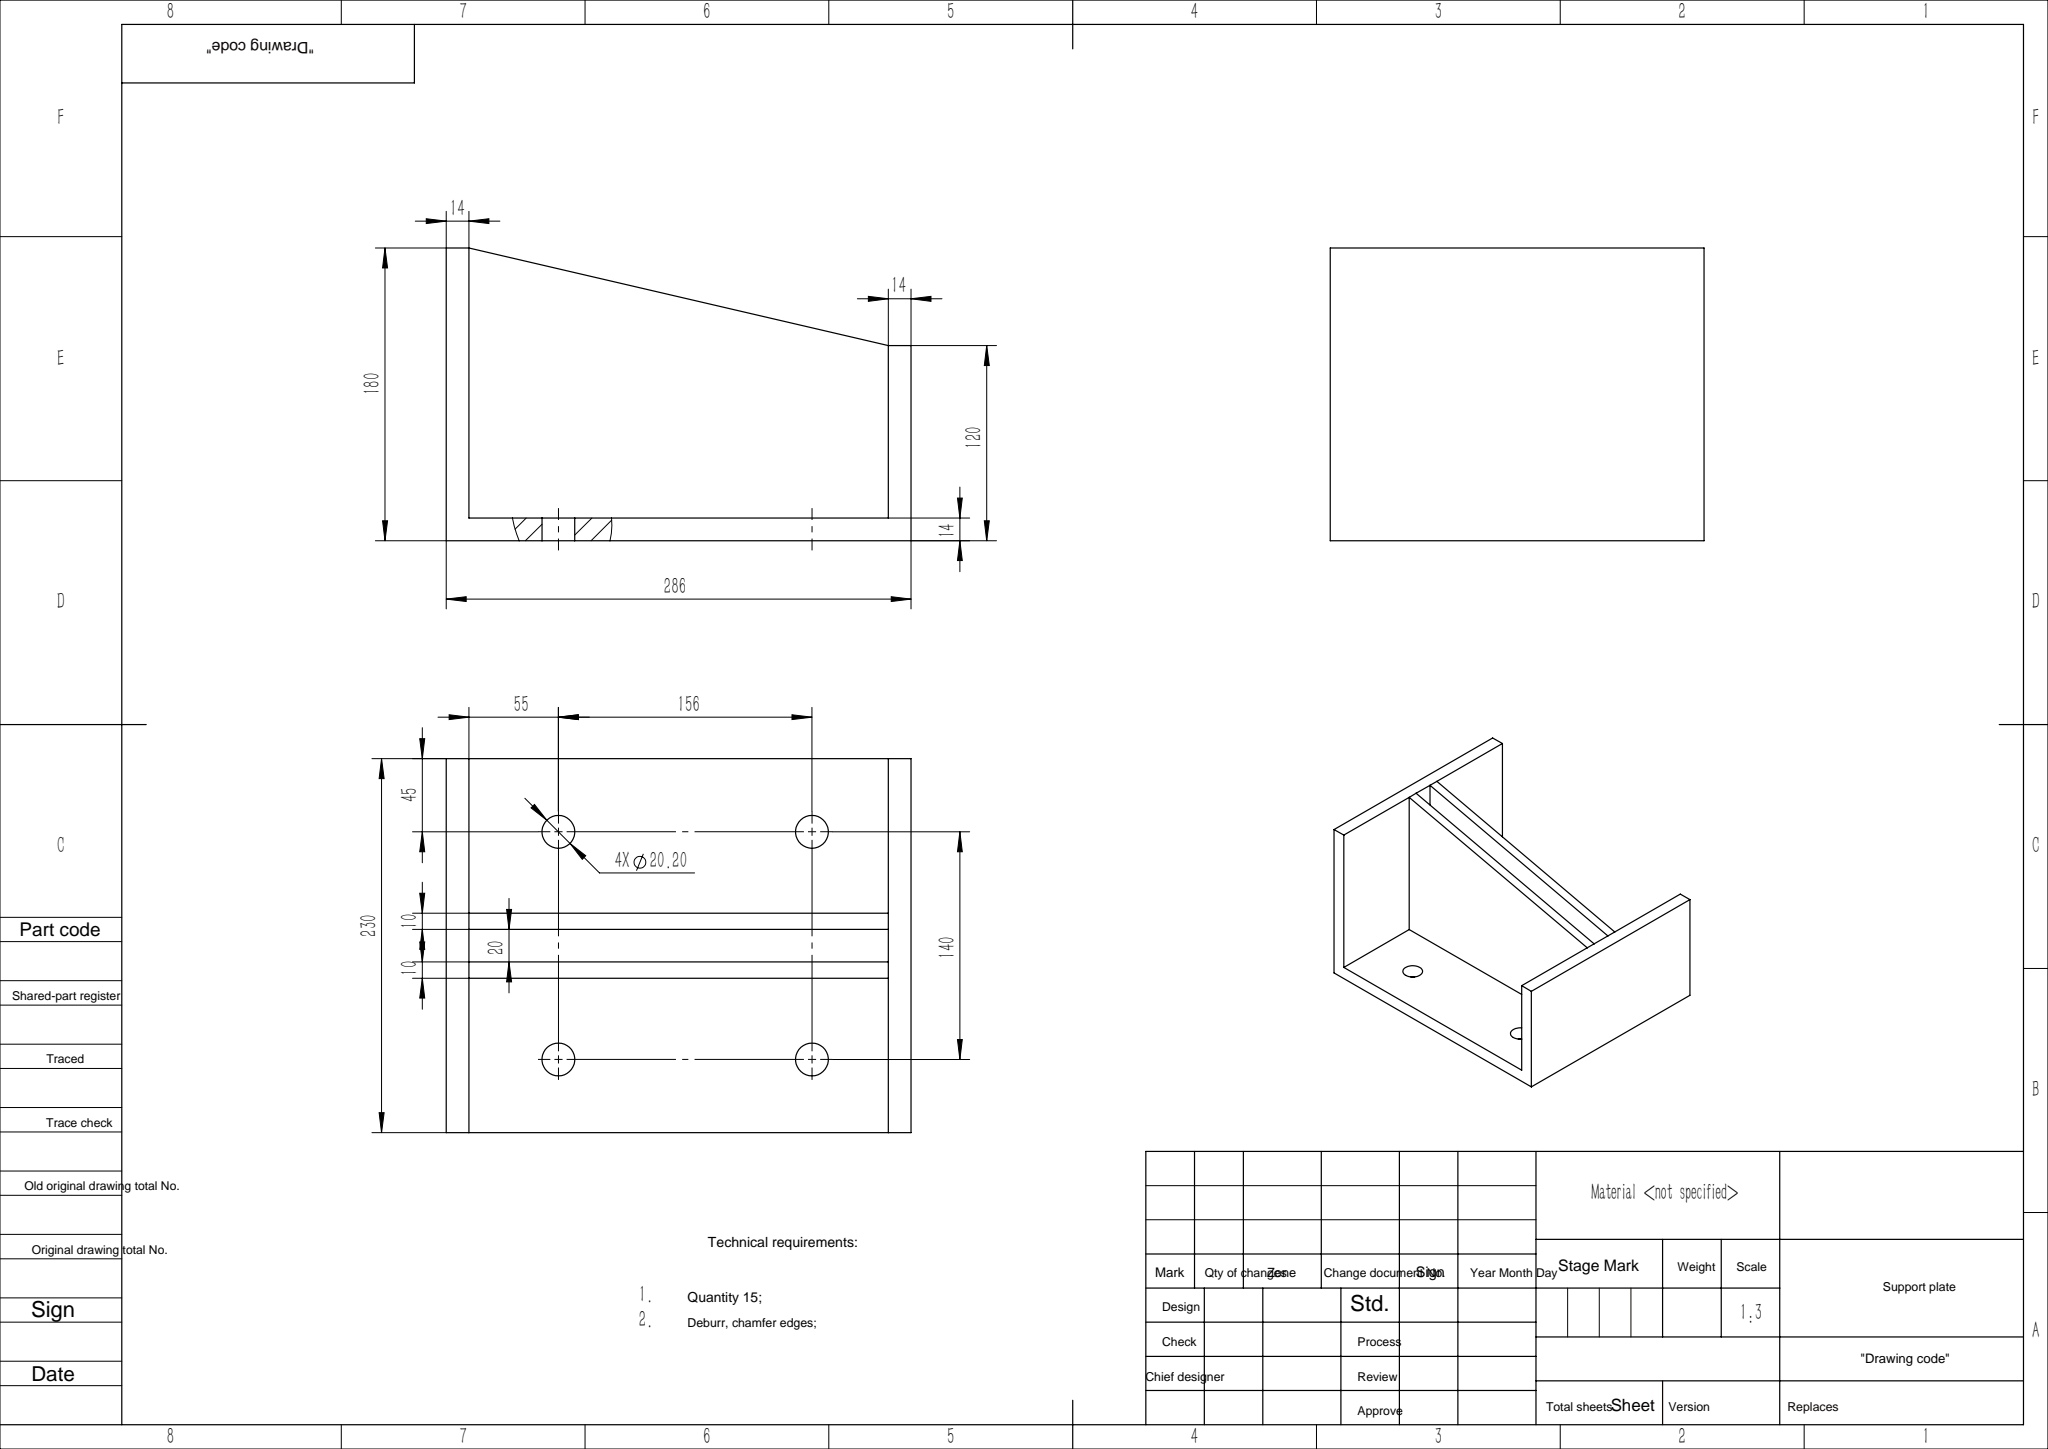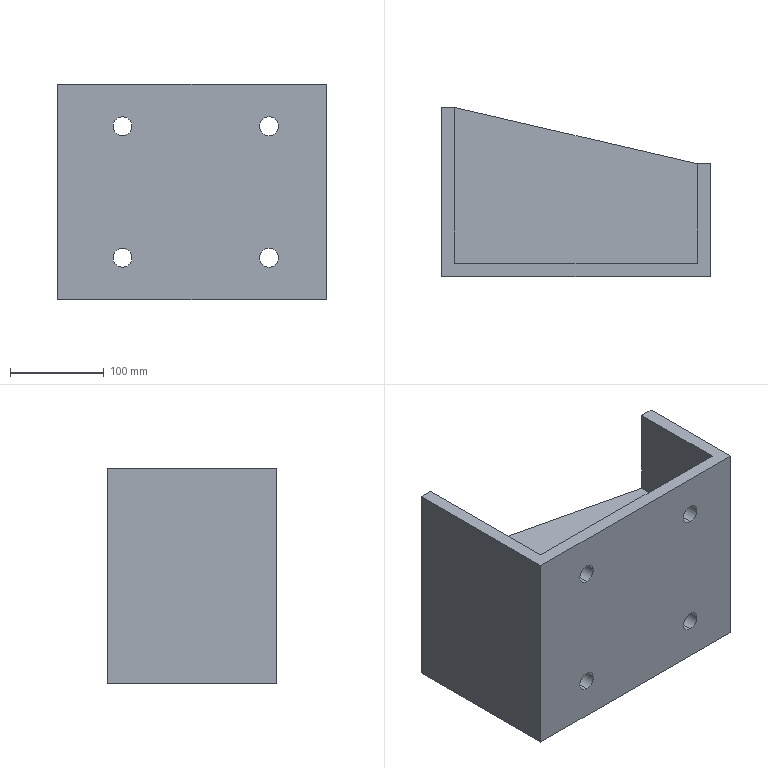Part | SolidWorks | features ICE 3, Extrusion 1, LPattern 1 | 1 solid | 30 faces | box 286 x 180 x 230 mm | volume 2480573 mm3 | plane 22 | cylinder 8 | commonest cylinder face diameters 20.2 x8
STEP:
#1=CARTESIAN_POINT('',(82.,0.,59.9));
#2=VERTEX_POINT('',#1);
#3=CARTESIAN_POINT('',(82.,0.,80.1));
#4=VERTEX_POINT('',#3);
#5=CARTESIAN_POINT('',(82.,0.,70.));
#6=DIRECTION('',(0.,1.,0.));
#7=DIRECTION('',(0.,0.,1.));
#8=AXIS2_PLACEMENT_3D('',#5,#6,#7);
#9=CIRCLE('',#8,10.1);
#10=EDGE_CURVE('',#2,#4,#9,.T.);
#11=ORIENTED_EDGE('',*,*,#10,.F.);
#12=CARTESIAN_POINT('',(82.,14.,59.9));
#13=VERTEX_POINT('',#12);
#14=CARTESIAN_POINT('',(82.,0.,59.9));
#15=DIRECTION('',(0.,1.,0.));
#16=VECTOR('',#15,1000.);
#17=LINE('',#14,#16);
#18=EDGE_CURVE('',#2,#13,#17,.T.);
#19=ORIENTED_EDGE('',*,*,#18,.T.);
#20=CARTESIAN_POINT('',(82.,14.,80.1));
#21=VERTEX_POINT('',#20);
#22=CARTESIAN_POINT('',(82.,14.,70.));
#23=DIRECTION('',(0.,1.,0.));
#24=DIRECTION('',(0.,0.,1.));
#25=AXIS2_PLACEMENT_3D('',#22,#23,#24);
#26=CIRCLE('',#25,10.1);
#27=EDGE_CURVE('',#13,#21,#26,.T.);
#28=ORIENTED_EDGE('',*,*,#27,.T.);
#29=CARTESIAN_POINT('',(82.,0.,80.1));
#30=DIRECTION('',(0.,1.,0.));
#31=VECTOR('',#30,1000.);
#32=LINE('',#29,#31);
#33=EDGE_CURVE('',#4,#21,#32,.T.);
#34=ORIENTED_EDGE('',*,*,#33,.F.);
#35=EDGE_LOOP('',(#11,#19,#28,#34));
#36=FACE_OUTER_BOUND('',#35,.T.);
#37=CARTESIAN_POINT('',(82.,0.,70.));
#38=DIRECTION('',(0.,1.,0.));
#39=DIRECTION('',(0.,0.,1.));
#40=AXIS2_PLACEMENT_3D('',#37,#38,#39);
#41=CYLINDRICAL_SURFACE('',#40,10.1);
#42=ADVANCED_FACE('',(#36),#41,.F.);
#43=CARTESIAN_POINT('',(82.,0.,-80.1));
#44=VERTEX_POINT('',#43);
#45=CARTESIAN_POINT('',(82.,0.,-59.9));
#46=VERTEX_POINT('',#45);
#47=CARTESIAN_POINT('',(82.,0.,-70.));
#48=DIRECTION('',(0.,1.,0.));
#49=DIRECTION('',(0.,0.,1.));
#50=AXIS2_PLACEMENT_3D('',#47,#48,#49);
#51=CIRCLE('',#50,10.1);
#52=EDGE_CURVE('',#44,#46,#51,.T.);
#53=ORIENTED_EDGE('',*,*,#52,.F.);
#54=CARTESIAN_POINT('',(82.,14.,-80.1));
#55=VERTEX_POINT('',#54);
#56=CARTESIAN_POINT('',(82.,0.,-80.1));
#57=DIRECTION('',(0.,1.,0.));
#58=VECTOR('',#57,1000.);
#59=LINE('',#56,#58);
#60=EDGE_CURVE('',#44,#55,#59,.T.);
#61=ORIENTED_EDGE('',*,*,#60,.T.);
#62=CARTESIAN_POINT('',(82.,14.,-59.9));
#63=VERTEX_POINT('',#62);
#64=CARTESIAN_POINT('',(82.,14.,-70.));
#65=DIRECTION('',(0.,1.,0.));
#66=DIRECTION('',(0.,0.,1.));
#67=AXIS2_PLACEMENT_3D('',#64,#65,#66);
#68=CIRCLE('',#67,10.1);
#69=EDGE_CURVE('',#55,#63,#68,.T.);
#70=ORIENTED_EDGE('',*,*,#69,.T.);
#71=CARTESIAN_POINT('',(82.,0.,-59.9));
#72=DIRECTION('',(0.,1.,0.));
#73=VECTOR('',#72,1000.);
#74=LINE('',#71,#73);
#75=EDGE_CURVE('',#46,#63,#74,.T.);
#76=ORIENTED_EDGE('',*,*,#75,.F.);
#77=EDGE_LOOP('',(#53,#61,#70,#76));
#78=FACE_OUTER_BOUND('',#77,.T.);
#79=CARTESIAN_POINT('',(82.,0.,-70.));
#80=DIRECTION('',(0.,1.,0.));
#81=DIRECTION('',(0.,0.,1.));
#82=AXIS2_PLACEMENT_3D('',#79,#80,#81);
#83=CYLINDRICAL_SURFACE('',#82,10.1);
#84=ADVANCED_FACE('',(#78),#83,.F.);
#85=CARTESIAN_POINT('',(-74.,0.,-80.1));
#86=VERTEX_POINT('',#85);
#87=CARTESIAN_POINT('',(-74.,0.,-59.9));
#88=VERTEX_POINT('',#87);
#89=CARTESIAN_POINT('',(-74.,0.,-70.));
#90=DIRECTION('',(0.,1.,0.));
#91=DIRECTION('',(0.,0.,1.));
#92=AXIS2_PLACEMENT_3D('',#89,#90,#91);
#93=CIRCLE('',#92,10.1);
#94=EDGE_CURVE('',#86,#88,#93,.T.);
#95=ORIENTED_EDGE('',*,*,#94,.F.);
#96=CARTESIAN_POINT('',(-74.,14.,-80.1));
#97=VERTEX_POINT('',#96);
#98=CARTESIAN_POINT('',(-74.,0.,-80.1));
#99=DIRECTION('',(0.,1.,0.));
#100=VECTOR('',#99,1000.);
#101=LINE('',#98,#100);
#102=EDGE_CURVE('',#86,#97,#101,.T.);
#103=ORIENTED_EDGE('',*,*,#102,.T.);
#104=CARTESIAN_POINT('',(-74.,14.,-59.9));
#105=VERTEX_POINT('',#104);
#106=CARTESIAN_POINT('',(-74.,14.,-70.));
#107=DIRECTION('',(0.,1.,0.));
#108=DIRECTION('',(0.,0.,1.));
#109=AXIS2_PLACEMENT_3D('',#106,#107,#108);
#110=CIRCLE('',#109,10.1);
#111=EDGE_CURVE('',#97,#105,#110,.T.);
#112=ORIENTED_EDGE('',*,*,#111,.T.);
#113=CARTESIAN_POINT('',(-74.,0.,-59.9));
#114=DIRECTION('',(0.,1.,0.));
#115=VECTOR('',#114,1000.);
#116=LINE('',#113,#115);
#117=EDGE_CURVE('',#88,#105,#116,.T.);
#118=ORIENTED_EDGE('',*,*,#117,.F.);
#119=EDGE_LOOP('',(#95,#103,#112,#118));
#120=FACE_OUTER_BOUND('',#119,.T.);
#121=CARTESIAN_POINT('',(-74.,0.,-70.));
#122=DIRECTION('',(0.,1.,0.));
#123=DIRECTION('',(0.,0.,1.));
#124=AXIS2_PLACEMENT_3D('',#121,#122,#123);
#125=CYLINDRICAL_SURFACE('',#124,10.1);
#126=ADVANCED_FACE('',(#120),#125,.F.);
#127=CARTESIAN_POINT('',(-74.,0.,59.9));
#128=VERTEX_POINT('',#127);
#129=CARTESIAN_POINT('',(-74.,0.,80.1));
#130=VERTEX_POINT('',#129);
#131=CARTESIAN_POINT('',(-74.,0.,70.));
#132=DIRECTION('',(0.,1.,0.));
#133=DIRECTION('',(0.,0.,1.));
#134=AXIS2_PLACEMENT_3D('',#131,#132,#133);
#135=CIRCLE('',#134,10.1);
#136=EDGE_CURVE('',#128,#130,#135,.T.);
#137=ORIENTED_EDGE('',*,*,#136,.F.);
#138=CARTESIAN_POINT('',(-74.,14.,59.9));
#139=VERTEX_POINT('',#138);
#140=CARTESIAN_POINT('',(-74.,0.,59.9));
#141=DIRECTION('',(0.,1.,0.));
#142=VECTOR('',#141,1000.);
#143=LINE('',#140,#142);
#144=EDGE_CURVE('',#128,#139,#143,.T.);
#145=ORIENTED_EDGE('',*,*,#144,.T.);
#146=CARTESIAN_POINT('',(-74.,14.,80.1));
#147=VERTEX_POINT('',#146);
#148=CARTESIAN_POINT('',(-74.,14.,70.));
#149=DIRECTION('',(0.,1.,0.));
#150=DIRECTION('',(0.,0.,1.));
#151=AXIS2_PLACEMENT_3D('',#148,#149,#150);
#152=CIRCLE('',#151,10.1);
#153=EDGE_CURVE('',#139,#147,#152,.T.);
#154=ORIENTED_EDGE('',*,*,#153,.T.);
#155=CARTESIAN_POINT('',(-74.,0.,80.1));
#156=DIRECTION('',(0.,1.,0.));
#157=VECTOR('',#156,1000.);
#158=LINE('',#155,#157);
#159=EDGE_CURVE('',#130,#147,#158,.T.);
#160=ORIENTED_EDGE('',*,*,#159,.F.);
#161=EDGE_LOOP('',(#137,#145,#154,#160));
#162=FACE_OUTER_BOUND('',#161,.T.);
#163=CARTESIAN_POINT('',(-74.,0.,70.));
#164=DIRECTION('',(0.,1.,0.));
#165=DIRECTION('',(0.,0.,1.));
#166=AXIS2_PLACEMENT_3D('',#163,#164,#165);
#167=CYLINDRICAL_SURFACE('',#166,10.1);
#168=ADVANCED_FACE('',(#162),#167,.F.);
#169=CARTESIAN_POINT('',(129.,14.,10.));
#170=VERTEX_POINT('',#169);
#171=CARTESIAN_POINT('',(129.,120.,10.));
#172=VERTEX_POINT('',#171);
#173=CARTESIAN_POINT('',(129.,14.,10.));
#174=DIRECTION('',(0.,1.,0.));
#175=VECTOR('',#174,1000.);
#176=LINE('',#173,#175);
#177=EDGE_CURVE('',#170,#172,#176,.T.);
#178=ORIENTED_EDGE('',*,*,#177,.T.);
#179=CARTESIAN_POINT('',(129.,120.,-10.));
#180=VERTEX_POINT('',#179);
#181=CARTESIAN_POINT('',(129.,120.,115.));
#182=DIRECTION('',(0.,0.,-1.));
#183=VECTOR('',#182,1000.);
#184=LINE('',#181,#183);
#185=EDGE_CURVE('',#172,#180,#184,.T.);
#186=ORIENTED_EDGE('',*,*,#185,.T.);
#187=CARTESIAN_POINT('',(129.,14.,-10.));
#188=VERTEX_POINT('',#187);
#189=CARTESIAN_POINT('',(129.,120.,-10.));
#190=DIRECTION('',(0.,1.,0.));
#191=VECTOR('',#190,1000.);
#192=LINE('',#189,#191);
#193=EDGE_CURVE('',#188,#180,#192,.T.);
#194=ORIENTED_EDGE('',*,*,#193,.F.);
#195=CARTESIAN_POINT('',(129.,14.,115.));
#196=DIRECTION('',(0.,0.,-1.));
#197=VECTOR('',#196,1000.);
#198=LINE('',#195,#197);
#199=EDGE_CURVE('',#170,#188,#198,.T.);
#200=ORIENTED_EDGE('',*,*,#199,.F.);
#201=EDGE_LOOP('',(#178,#186,#194,#200));
#202=FACE_OUTER_BOUND('',#201,.T.);
#203=CARTESIAN_POINT('',(129.,14.,115.));
#204=DIRECTION('',(1.,0.,0.));
#205=DIRECTION('',(0.,1.,0.));
#206=AXIS2_PLACEMENT_3D('',#203,#204,#205);
#207=PLANE('',#206);
#208=ADVANCED_FACE('',(#202),#207,.F.);
#209=CARTESIAN_POINT('',(-129.,14.,10.));
#210=VERTEX_POINT('',#209);
#211=CARTESIAN_POINT('',(-129.,14.,10.));
#212=DIRECTION('',(1.,0.,0.));
#213=VECTOR('',#212,1000.);
#214=LINE('',#211,#213);
#215=EDGE_CURVE('',#210,#170,#214,.T.);
#216=ORIENTED_EDGE('',*,*,#215,.T.);
#217=ORIENTED_EDGE('',*,*,#199,.T.);
#218=CARTESIAN_POINT('',(-129.,14.,-10.));
#219=VERTEX_POINT('',#218);
#220=CARTESIAN_POINT('',(129.,14.,-10.));
#221=DIRECTION('',(1.,0.,0.));
#222=VECTOR('',#221,1000.);
#223=LINE('',#220,#222);
#224=EDGE_CURVE('',#219,#188,#223,.T.);
#225=ORIENTED_EDGE('',*,*,#224,.F.);
#226=CARTESIAN_POINT('',(-129.,14.,115.));
#227=DIRECTION('',(0.,0.,-1.));
#228=VECTOR('',#227,1000.);
#229=LINE('',#226,#228);
#230=EDGE_CURVE('',#210,#219,#229,.T.);
#231=ORIENTED_EDGE('',*,*,#230,.F.);
#232=EDGE_LOOP('',(#216,#217,#225,#231));
#233=FACE_OUTER_BOUND('',#232,.T.);
#234=CARTESIAN_POINT('',(-129.,14.,115.));
#235=DIRECTION('',(0.,-1.,0.));
#236=DIRECTION('',(0.,0.,-1.));
#237=AXIS2_PLACEMENT_3D('',#234,#235,#236);
#238=PLANE('',#237);
#239=ADVANCED_FACE('',(#233),#238,.F.);
#240=CARTESIAN_POINT('',(-129.,180.,10.));
#241=VERTEX_POINT('',#240);
#242=CARTESIAN_POINT('',(-129.,180.,10.));
#243=DIRECTION('',(0.,-1.,0.));
#244=VECTOR('',#243,1000.);
#245=LINE('',#242,#244);
#246=EDGE_CURVE('',#241,#210,#245,.T.);
#247=ORIENTED_EDGE('',*,*,#246,.T.);
#248=ORIENTED_EDGE('',*,*,#230,.T.);
#249=CARTESIAN_POINT('',(-129.,180.,-10.));
#250=VERTEX_POINT('',#249);
#251=CARTESIAN_POINT('',(-129.,14.,-10.));
#252=DIRECTION('',(0.,-1.,0.));
#253=VECTOR('',#252,1000.);
#254=LINE('',#251,#253);
#255=EDGE_CURVE('',#250,#219,#254,.T.);
#256=ORIENTED_EDGE('',*,*,#255,.F.);
#257=CARTESIAN_POINT('',(-129.,180.,115.));
#258=DIRECTION('',(0.,0.,-1.));
#259=VECTOR('',#258,1000.);
#260=LINE('',#257,#259);
#261=EDGE_CURVE('',#241,#250,#260,.T.);
#262=ORIENTED_EDGE('',*,*,#261,.F.);
#263=EDGE_LOOP('',(#247,#248,#256,#262));
#264=FACE_OUTER_BOUND('',#263,.T.);
#265=CARTESIAN_POINT('',(-129.,180.,115.));
#266=DIRECTION('',(-1.,0.,0.));
#267=DIRECTION('',(0.,-1.,0.));
#268=AXIS2_PLACEMENT_3D('',#265,#266,#267);
#269=PLANE('',#268);
#270=ADVANCED_FACE('',(#264),#269,.F.);
#271=CARTESIAN_POINT('',(129.,120.,115.));
#272=VERTEX_POINT('',#271);
#273=CARTESIAN_POINT('',(129.,120.,20.));
#274=VERTEX_POINT('',#273);
#275=CARTESIAN_POINT('',(129.,120.,115.));
#276=DIRECTION('',(0.,0.,-1.));
#277=VECTOR('',#276,1000.);
#278=LINE('',#275,#277);
#279=EDGE_CURVE('',#272,#274,#278,.T.);
#280=ORIENTED_EDGE('',*,*,#279,.T.);
#281=CARTESIAN_POINT('',(129.,14.,20.));
#282=VERTEX_POINT('',#281);
#283=CARTESIAN_POINT('',(129.,14.,20.));
#284=DIRECTION('',(0.,1.,0.));
#285=VECTOR('',#284,1000.);
#286=LINE('',#283,#285);
#287=EDGE_CURVE('',#282,#274,#286,.T.);
#288=ORIENTED_EDGE('',*,*,#287,.F.);
#289=CARTESIAN_POINT('',(129.,14.,115.));
#290=VERTEX_POINT('',#289);
#291=CARTESIAN_POINT('',(129.,14.,115.));
#292=DIRECTION('',(0.,0.,-1.));
#293=VECTOR('',#292,1000.);
#294=LINE('',#291,#293);
#295=EDGE_CURVE('',#290,#282,#294,.T.);
#296=ORIENTED_EDGE('',*,*,#295,.F.);
#297=CARTESIAN_POINT('',(129.,14.,115.));
#298=DIRECTION('',(0.,-1.,0.));
#299=VECTOR('',#298,1000.);
#300=LINE('',#297,#299);
#301=EDGE_CURVE('',#272,#290,#300,.T.);
#302=ORIENTED_EDGE('',*,*,#301,.F.);
#303=EDGE_LOOP('',(#280,#288,#296,#302));
#304=FACE_OUTER_BOUND('',#303,.T.);
#305=CARTESIAN_POINT('',(129.,14.,115.));
#306=DIRECTION('',(1.,0.,0.));
#307=DIRECTION('',(0.,1.,0.));
#308=AXIS2_PLACEMENT_3D('',#305,#306,#307);
#309=PLANE('',#308);
#310=ADVANCED_FACE('',(#304),#309,.F.);
#311=CARTESIAN_POINT('',(82.,14.,70.));
#312=DIRECTION('',(0.,1.,0.));
#313=DIRECTION('',(0.,0.,1.));
#314=AXIS2_PLACEMENT_3D('',#311,#312,#313);
#315=CIRCLE('',#314,10.1);
#316=EDGE_CURVE('',#21,#13,#315,.T.);
#317=ORIENTED_EDGE('',*,*,#316,.F.);
#318=ORIENTED_EDGE('',*,*,#27,.F.);
#319=EDGE_LOOP('',(#317,#318));
#320=FACE_BOUND('',#319,.T.);
#321=CARTESIAN_POINT('',(-74.,14.,70.));
#322=DIRECTION('',(0.,1.,0.));
#323=DIRECTION('',(0.,0.,1.));
#324=AXIS2_PLACEMENT_3D('',#321,#322,#323);
#325=CIRCLE('',#324,10.1);
#326=EDGE_CURVE('',#147,#139,#325,.T.);
#327=ORIENTED_EDGE('',*,*,#326,.F.);
#328=ORIENTED_EDGE('',*,*,#153,.F.);
#329=EDGE_LOOP('',(#327,#328));
#330=FACE_BOUND('',#329,.T.);
#331=ORIENTED_EDGE('',*,*,#295,.T.);
#332=CARTESIAN_POINT('',(-129.,14.,20.));
#333=VERTEX_POINT('',#332);
#334=CARTESIAN_POINT('',(-129.,14.,20.));
#335=DIRECTION('',(1.,0.,0.));
#336=VECTOR('',#335,1000.);
#337=LINE('',#334,#336);
#338=EDGE_CURVE('',#333,#282,#337,.T.);
#339=ORIENTED_EDGE('',*,*,#338,.F.);
#340=CARTESIAN_POINT('',(-129.,14.,115.));
#341=VERTEX_POINT('',#340);
#342=CARTESIAN_POINT('',(-129.,14.,115.));
#343=DIRECTION('',(0.,0.,-1.));
#344=VECTOR('',#343,1000.);
#345=LINE('',#342,#344);
#346=EDGE_CURVE('',#341,#333,#345,.T.);
#347=ORIENTED_EDGE('',*,*,#346,.F.);
#348=CARTESIAN_POINT('',(-129.,14.,115.));
#349=DIRECTION('',(-1.,0.,0.));
#350=VECTOR('',#349,1000.);
#351=LINE('',#348,#350);
#352=EDGE_CURVE('',#290,#341,#351,.T.);
#353=ORIENTED_EDGE('',*,*,#352,.F.);
#354=EDGE_LOOP('',(#331,#339,#347,#353));
#355=FACE_OUTER_BOUND('',#354,.T.);
#356=CARTESIAN_POINT('',(-129.,14.,115.));
#357=DIRECTION('',(0.,-1.,0.));
#358=DIRECTION('',(0.,0.,-1.));
#359=AXIS2_PLACEMENT_3D('',#356,#357,#358);
#360=PLANE('',#359);
#361=ADVANCED_FACE('',(#320,#330,#355),#360,.F.);
#362=ORIENTED_EDGE('',*,*,#346,.T.);
#363=CARTESIAN_POINT('',(-129.,180.,20.));
#364=VERTEX_POINT('',#363);
#365=CARTESIAN_POINT('',(-129.,180.,20.));
#366=DIRECTION('',(0.,-1.,0.));
#367=VECTOR('',#366,1000.);
#368=LINE('',#365,#367);
#369=EDGE_CURVE('',#364,#333,#368,.T.);
#370=ORIENTED_EDGE('',*,*,#369,.F.);
#371=CARTESIAN_POINT('',(-129.,180.,115.));
#372=VERTEX_POINT('',#371);
#373=CARTESIAN_POINT('',(-129.,180.,115.));
#374=DIRECTION('',(0.,0.,-1.));
#375=VECTOR('',#374,1000.);
#376=LINE('',#373,#375);
#377=EDGE_CURVE('',#372,#364,#376,.T.);
#378=ORIENTED_EDGE('',*,*,#377,.F.);
#379=CARTESIAN_POINT('',(-129.,180.,115.));
#380=DIRECTION('',(0.,1.,0.));
#381=VECTOR('',#380,1000.);
#382=LINE('',#379,#381);
#383=EDGE_CURVE('',#341,#372,#382,.T.);
#384=ORIENTED_EDGE('',*,*,#383,.F.);
#385=EDGE_LOOP('',(#362,#370,#378,#384));
#386=FACE_OUTER_BOUND('',#385,.T.);
#387=CARTESIAN_POINT('',(-129.,180.,115.));
#388=DIRECTION('',(-1.,0.,0.));
#389=DIRECTION('',(0.,-1.,0.));
#390=AXIS2_PLACEMENT_3D('',#387,#388,#389);
#391=PLANE('',#390);
#392=ADVANCED_FACE('',(#386),#391,.F.);
#393=CARTESIAN_POINT('',(-143.,180.,-115.));
#394=VERTEX_POINT('',#393);
#395=CARTESIAN_POINT('',(-143.,0.,-115.));
#396=VERTEX_POINT('',#395);
#397=CARTESIAN_POINT('',(-143.,180.,-115.));
#398=DIRECTION('',(0.,-1.,0.));
#399=VECTOR('',#398,1000.);
#400=LINE('',#397,#399);
#401=EDGE_CURVE('',#394,#396,#400,.T.);
#402=ORIENTED_EDGE('',*,*,#401,.T.);
#403=CARTESIAN_POINT('',(-143.,0.,115.));
#404=VERTEX_POINT('',#403);
#405=CARTESIAN_POINT('',(-143.,0.,115.));
#406=DIRECTION('',(0.,0.,-1.));
#407=VECTOR('',#406,1000.);
#408=LINE('',#405,#407);
#409=EDGE_CURVE('',#404,#396,#408,.T.);
#410=ORIENTED_EDGE('',*,*,#409,.F.);
#411=CARTESIAN_POINT('',(-143.,180.,115.));
#412=VERTEX_POINT('',#411);
#413=CARTESIAN_POINT('',(-143.,180.,115.));
#414=DIRECTION('',(0.,-1.,0.));
#415=VECTOR('',#414,1000.);
#416=LINE('',#413,#415);
#417=EDGE_CURVE('',#412,#404,#416,.T.);
#418=ORIENTED_EDGE('',*,*,#417,.F.);
#419=CARTESIAN_POINT('',(-143.,180.,115.));
#420=DIRECTION('',(0.,0.,-1.));
#421=VECTOR('',#420,1000.);
#422=LINE('',#419,#421);
#423=EDGE_CURVE('',#412,#394,#422,.T.);
#424=ORIENTED_EDGE('',*,*,#423,.T.);
#425=EDGE_LOOP('',(#402,#410,#418,#424));
#426=FACE_OUTER_BOUND('',#425,.T.);
#427=CARTESIAN_POINT('',(-143.,180.,115.));
#428=DIRECTION('',(1.,0.,0.));
#429=DIRECTION('',(0.,1.,0.));
#430=AXIS2_PLACEMENT_3D('',#427,#428,#429);
#431=PLANE('',#430);
#432=ADVANCED_FACE('',(#426),#431,.F.);
#433=CARTESIAN_POINT('',(82.,0.,70.));
#434=DIRECTION('',(0.,1.,0.));
#435=DIRECTION('',(0.,0.,1.));
#436=AXIS2_PLACEMENT_3D('',#433,#434,#435);
#437=CIRCLE('',#436,10.1);
#438=EDGE_CURVE('',#4,#2,#437,.T.);
#439=ORIENTED_EDGE('',*,*,#438,.T.);
#440=ORIENTED_EDGE('',*,*,#10,.T.);
#441=EDGE_LOOP('',(#439,#440));
#442=FACE_BOUND('',#441,.T.);
#443=CARTESIAN_POINT('',(82.,0.,-70.));
#444=DIRECTION('',(0.,1.,0.));
#445=DIRECTION('',(0.,0.,1.));
#446=AXIS2_PLACEMENT_3D('',#443,#444,#445);
#447=CIRCLE('',#446,10.1);
#448=EDGE_CURVE('',#46,#44,#447,.T.);
#449=ORIENTED_EDGE('',*,*,#448,.T.);
#450=ORIENTED_EDGE('',*,*,#52,.T.);
#451=EDGE_LOOP('',(#449,#450));
#452=FACE_BOUND('',#451,.T.);
#453=CARTESIAN_POINT('',(-74.,0.,-70.));
#454=DIRECTION('',(0.,1.,0.));
#455=DIRECTION('',(0.,0.,1.));
#456=AXIS2_PLACEMENT_3D('',#453,#454,#455);
#457=CIRCLE('',#456,10.1);
#458=EDGE_CURVE('',#88,#86,#457,.T.);
#459=ORIENTED_EDGE('',*,*,#458,.T.);
#460=ORIENTED_EDGE('',*,*,#94,.T.);
#461=EDGE_LOOP('',(#459,#460));
#462=FACE_BOUND('',#461,.T.);
#463=CARTESIAN_POINT('',(-74.,0.,70.));
#464=DIRECTION('',(0.,1.,0.));
#465=DIRECTION('',(0.,0.,1.));
#466=AXIS2_PLACEMENT_3D('',#463,#464,#465);
#467=CIRCLE('',#466,10.1);
#468=EDGE_CURVE('',#130,#128,#467,.T.);
#469=ORIENTED_EDGE('',*,*,#468,.T.);
#470=ORIENTED_EDGE('',*,*,#136,.T.);
#471=EDGE_LOOP('',(#469,#470));
#472=FACE_BOUND('',#471,.T.);
#473=CARTESIAN_POINT('',(143.,0.,-115.));
#474=VERTEX_POINT('',#473);
#475=CARTESIAN_POINT('',(-143.,0.,-115.));
#476=DIRECTION('',(1.,0.,0.));
#477=VECTOR('',#476,1000.);
#478=LINE('',#475,#477);
#479=EDGE_CURVE('',#396,#474,#478,.T.);
#480=ORIENTED_EDGE('',*,*,#479,.T.);
#481=CARTESIAN_POINT('',(143.,0.,115.));
#482=VERTEX_POINT('',#481);
#483=CARTESIAN_POINT('',(143.,0.,115.));
#484=DIRECTION('',(0.,0.,-1.));
#485=VECTOR('',#484,1000.);
#486=LINE('',#483,#485);
#487=EDGE_CURVE('',#482,#474,#486,.T.);
#488=ORIENTED_EDGE('',*,*,#487,.F.);
#489=CARTESIAN_POINT('',(-143.,0.,115.));
#490=DIRECTION('',(1.,0.,0.));
#491=VECTOR('',#490,1000.);
#492=LINE('',#489,#491);
#493=EDGE_CURVE('',#404,#482,#492,.T.);
#494=ORIENTED_EDGE('',*,*,#493,.F.);
#495=ORIENTED_EDGE('',*,*,#409,.T.);
#496=EDGE_LOOP('',(#480,#488,#494,#495));
#497=FACE_OUTER_BOUND('',#496,.T.);
#498=CARTESIAN_POINT('',(-143.,0.,115.));
#499=DIRECTION('',(0.,1.,0.));
#500=DIRECTION('',(0.,0.,1.));
#501=AXIS2_PLACEMENT_3D('',#498,#499,#500);
#502=PLANE('',#501);
#503=ADVANCED_FACE('',(#442,#452,#462,#472,#497),#502,.F.);
#504=CARTESIAN_POINT('',(143.,120.,-115.));
#505=VERTEX_POINT('',#504);
#506=CARTESIAN_POINT('',(143.,120.,-115.));
#507=DIRECTION('',(0.,1.,0.));
#508=VECTOR('',#507,1000.);
#509=LINE('',#506,#508);
#510=EDGE_CURVE('',#474,#505,#509,.T.);
#511=ORIENTED_EDGE('',*,*,#510,.T.);
#512=CARTESIAN_POINT('',(143.,120.,115.));
#513=VERTEX_POINT('',#512);
#514=CARTESIAN_POINT('',(143.,120.,115.));
#515=DIRECTION('',(0.,0.,-1.));
#516=VECTOR('',#515,1000.);
#517=LINE('',#514,#516);
#518=EDGE_CURVE('',#513,#505,#517,.T.);
#519=ORIENTED_EDGE('',*,*,#518,.F.);
#520=CARTESIAN_POINT('',(143.,120.,115.));
#521=DIRECTION('',(0.,1.,0.));
#522=VECTOR('',#521,1000.);
#523=LINE('',#520,#522);
#524=EDGE_CURVE('',#482,#513,#523,.T.);
#525=ORIENTED_EDGE('',*,*,#524,.F.);
#526=ORIENTED_EDGE('',*,*,#487,.T.);
#527=EDGE_LOOP('',(#511,#519,#525,#526));
#528=FACE_OUTER_BOUND('',#527,.T.);
#529=CARTESIAN_POINT('',(143.,120.,115.));
#530=DIRECTION('',(-1.,0.,0.));
#531=DIRECTION('',(0.,-1.,0.));
#532=AXIS2_PLACEMENT_3D('',#529,#530,#531);
#533=PLANE('',#532);
#534=ADVANCED_FACE('',(#528),#533,.F.);
#535=CARTESIAN_POINT('',(129.,120.,-115.));
#536=VERTEX_POINT('',#535);
#537=CARTESIAN_POINT('',(129.,120.,-115.));
#538=DIRECTION('',(-1.,0.,0.));
#539=VECTOR('',#538,1000.);
#540=LINE('',#537,#539);
#541=EDGE_CURVE('',#505,#536,#540,.T.);
#542=ORIENTED_EDGE('',*,*,#541,.T.);
#543=CARTESIAN_POINT('',(129.,120.,-20.));
#544=VERTEX_POINT('',#543);
#545=CARTESIAN_POINT('',(129.,120.,115.));
#546=DIRECTION('',(0.,0.,-1.));
#547=VECTOR('',#546,1000.);
#548=LINE('',#545,#547);
#549=EDGE_CURVE('',#544,#536,#548,.T.);
#550=ORIENTED_EDGE('',*,*,#549,.F.);
#551=CARTESIAN_POINT('',(129.,120.,-20.));
#552=DIRECTION('',(0.,0.,1.));
#553=VECTOR('',#552,1000.);
#554=LINE('',#551,#553);
#555=EDGE_CURVE('',#544,#180,#554,.T.);
#556=ORIENTED_EDGE('',*,*,#555,.T.);
#557=ORIENTED_EDGE('',*,*,#185,.F.);
#558=CARTESIAN_POINT('',(129.,120.,20.));
#559=DIRECTION('',(0.,0.,-1.));
#560=VECTOR('',#559,1000.);
#561=LINE('',#558,#560);
#562=EDGE_CURVE('',#274,#172,#561,.T.);
#563=ORIENTED_EDGE('',*,*,#562,.F.);
#564=ORIENTED_EDGE('',*,*,#279,.F.);
#565=CARTESIAN_POINT('',(129.,120.,115.));
#566=DIRECTION('',(-1.,0.,0.));
#567=VECTOR('',#566,1000.);
#568=LINE('',#565,#567);
#569=EDGE_CURVE('',#513,#272,#568,.T.);
#570=ORIENTED_EDGE('',*,*,#569,.F.);
#571=ORIENTED_EDGE('',*,*,#518,.T.);
#572=EDGE_LOOP('',(#542,#550,#556,#557,#563,#564,#570,#571));
#573=FACE_OUTER_BOUND('',#572,.T.);
#574=CARTESIAN_POINT('',(129.,120.,115.));
#575=DIRECTION('',(0.,-1.,0.));
#576=DIRECTION('',(0.,0.,-1.));
#577=AXIS2_PLACEMENT_3D('',#574,#575,#576);
#578=PLANE('',#577);
#579=ADVANCED_FACE('',(#573),#578,.F.);
#580=CARTESIAN_POINT('',(129.,14.,-20.));
#581=VERTEX_POINT('',#580);
#582=CARTESIAN_POINT('',(129.,14.,-115.));
#583=VERTEX_POINT('',#582);
#584=CARTESIAN_POINT('',(129.,14.,115.));
#585=DIRECTION('',(0.,0.,-1.));
#586=VECTOR('',#585,1000.);
#587=LINE('',#584,#586);
#588=EDGE_CURVE('',#581,#583,#587,.T.);
#589=ORIENTED_EDGE('',*,*,#588,.F.);
#590=CARTESIAN_POINT('',(129.,120.,-20.));
#591=DIRECTION('',(0.,1.,0.));
#592=VECTOR('',#591,1000.);
#593=LINE('',#590,#592);
#594=EDGE_CURVE('',#581,#544,#593,.T.);
#595=ORIENTED_EDGE('',*,*,#594,.T.);
#596=ORIENTED_EDGE('',*,*,#549,.T.);
#597=CARTESIAN_POINT('',(129.,14.,-115.));
#598=DIRECTION('',(0.,-1.,0.));
#599=VECTOR('',#598,1000.);
#600=LINE('',#597,#599);
#601=EDGE_CURVE('',#536,#583,#600,.T.);
#602=ORIENTED_EDGE('',*,*,#601,.T.);
#603=EDGE_LOOP('',(#589,#595,#596,#602));
#604=FACE_OUTER_BOUND('',#603,.T.);
#605=CARTESIAN_POINT('',(129.,14.,115.));
#606=DIRECTION('',(1.,0.,0.));
#607=DIRECTION('',(0.,1.,0.));
#608=AXIS2_PLACEMENT_3D('',#605,#606,#607);
#609=PLANE('',#608);
#610=ADVANCED_FACE('',(#604),#609,.F.);
#611=CARTESIAN_POINT('',(82.,14.,-70.));
#612=DIRECTION('',(0.,1.,0.));
#613=DIRECTION('',(0.,0.,1.));
#614=AXIS2_PLACEMENT_3D('',#611,#612,#613);
#615=CIRCLE('',#614,10.1);
#616=EDGE_CURVE('',#63,#55,#615,.T.);
#617=ORIENTED_EDGE('',*,*,#616,.F.);
#618=ORIENTED_EDGE('',*,*,#69,.F.);
#619=EDGE_LOOP('',(#617,#618));
#620=FACE_BOUND('',#619,.T.);
#621=CARTESIAN_POINT('',(-74.,14.,-70.));
#622=DIRECTION('',(0.,1.,0.));
#623=DIRECTION('',(0.,0.,1.));
#624=AXIS2_PLACEMENT_3D('',#621,#622,#623);
#625=CIRCLE('',#624,10.1);
#626=EDGE_CURVE('',#105,#97,#625,.T.);
#627=ORIENTED_EDGE('',*,*,#626,.F.);
#628=ORIENTED_EDGE('',*,*,#111,.F.);
#629=EDGE_LOOP('',(#627,#628));
#630=FACE_BOUND('',#629,.T.);
#631=CARTESIAN_POINT('',(-129.,14.,-20.));
#632=VERTEX_POINT('',#631);
#633=CARTESIAN_POINT('',(-129.,14.,-115.));
#634=VERTEX_POINT('',#633);
#635=CARTESIAN_POINT('',(-129.,14.,115.));
#636=DIRECTION('',(0.,0.,-1.));
#637=VECTOR('',#636,1000.);
#638=LINE('',#635,#637);
#639=EDGE_CURVE('',#632,#634,#638,.T.);
#640=ORIENTED_EDGE('',*,*,#639,.F.);
#641=CARTESIAN_POINT('',(129.,14.,-20.));
#642=DIRECTION('',(1.,0.,0.));
#643=VECTOR('',#642,1000.);
#644=LINE('',#641,#643);
#645=EDGE_CURVE('',#632,#581,#644,.T.);
#646=ORIENTED_EDGE('',*,*,#645,.T.);
#647=ORIENTED_EDGE('',*,*,#588,.T.);
#648=CARTESIAN_POINT('',(-129.,14.,-115.));
#649=DIRECTION('',(-1.,0.,0.));
#650=VECTOR('',#649,1000.);
#651=LINE('',#648,#650);
#652=EDGE_CURVE('',#583,#634,#651,.T.);
#653=ORIENTED_EDGE('',*,*,#652,.T.);
#654=EDGE_LOOP('',(#640,#646,#647,#653));
#655=FACE_OUTER_BOUND('',#654,.T.);
#656=CARTESIAN_POINT('',(-129.,14.,115.));
#657=DIRECTION('',(0.,-1.,0.));
#658=DIRECTION('',(0.,0.,-1.));
#659=AXIS2_PLACEMENT_3D('',#656,#657,#658);
#660=PLANE('',#659);
#661=ADVANCED_FACE('',(#620,#630,#655),#660,.F.);
#662=CARTESIAN_POINT('',(-129.,180.,-20.));
#663=VERTEX_POINT('',#662);
#664=CARTESIAN_POINT('',(-129.,180.,-115.));
#665=VERTEX_POINT('',#664);
#666=CARTESIAN_POINT('',(-129.,180.,115.));
#667=DIRECTION('',(0.,0.,-1.));
#668=VECTOR('',#667,1000.);
#669=LINE('',#666,#668);
#670=EDGE_CURVE('',#663,#665,#669,.T.);
#671=ORIENTED_EDGE('',*,*,#670,.F.);
#672=CARTESIAN_POINT('',(-129.,14.,-20.));
#673=DIRECTION('',(0.,-1.,0.));
#674=VECTOR('',#673,1000.);
#675=LINE('',#672,#674);
#676=EDGE_CURVE('',#663,#632,#675,.T.);
#677=ORIENTED_EDGE('',*,*,#676,.T.);
#678=ORIENTED_EDGE('',*,*,#639,.T.);
#679=CARTESIAN_POINT('',(-129.,180.,-115.));
#680=DIRECTION('',(0.,1.,0.));
#681=VECTOR('',#680,1000.);
#682=LINE('',#679,#681);
#683=EDGE_CURVE('',#634,#665,#682,.T.);
#684=ORIENTED_EDGE('',*,*,#683,.T.);
#685=EDGE_LOOP('',(#671,#677,#678,#684));
#686=FACE_OUTER_BOUND('',#685,.T.);
#687=CARTESIAN_POINT('',(-129.,180.,115.));
#688=DIRECTION('',(-1.,0.,0.));
#689=DIRECTION('',(0.,-1.,0.));
#690=AXIS2_PLACEMENT_3D('',#687,#688,#689);
#691=PLANE('',#690);
#692=ADVANCED_FACE('',(#686),#691,.F.);
#693=CARTESIAN_POINT('',(-143.,180.,-115.));
#694=DIRECTION('',(-1.,0.,0.));
#695=VECTOR('',#694,1000.);
#696=LINE('',#693,#695);
#697=EDGE_CURVE('',#665,#394,#696,.T.);
#698=ORIENTED_EDGE('',*,*,#697,.T.);
#699=ORIENTED_EDGE('',*,*,#423,.F.);
#700=CARTESIAN_POINT('',(-143.,180.,115.));
#701=DIRECTION('',(-1.,0.,0.));
#702=VECTOR('',#701,1000.);
#703=LINE('',#700,#702);
#704=EDGE_CURVE('',#372,#412,#703,.T.);
#705=ORIENTED_EDGE('',*,*,#704,.F.);
#706=ORIENTED_EDGE('',*,*,#377,.T.);
#707=CARTESIAN_POINT('',(-129.,180.,20.));
#708=DIRECTION('',(0.,0.,-1.));
#709=VECTOR('',#708,1000.);
#710=LINE('',#707,#709);
#711=EDGE_CURVE('',#364,#241,#710,.T.);
#712=ORIENTED_EDGE('',*,*,#711,.T.);
#713=ORIENTED_EDGE('',*,*,#261,.T.);
#714=CARTESIAN_POINT('',(-129.,180.,-20.));
#715=DIRECTION('',(0.,0.,1.));
#716=VECTOR('',#715,1000.);
#717=LINE('',#714,#716);
#718=EDGE_CURVE('',#663,#250,#717,.T.);
#719=ORIENTED_EDGE('',*,*,#718,.F.);
#720=ORIENTED_EDGE('',*,*,#670,.T.);
#721=EDGE_LOOP('',(#698,#699,#705,#706,#712,#713,#719,#720));
#722=FACE_OUTER_BOUND('',#721,.T.);
#723=CARTESIAN_POINT('',(-143.,180.,115.));
#724=DIRECTION('',(0.,-1.,0.));
#725=DIRECTION('',(0.,0.,-1.));
#726=AXIS2_PLACEMENT_3D('',#723,#724,#725);
#727=PLANE('',#726);
#728=ADVANCED_FACE('',(#722),#727,.F.);
#729=ORIENTED_EDGE('',*,*,#417,.T.);
#730=ORIENTED_EDGE('',*,*,#493,.T.);
#731=ORIENTED_EDGE('',*,*,#524,.T.);
#732=ORIENTED_EDGE('',*,*,#569,.T.);
#733=ORIENTED_EDGE('',*,*,#301,.T.);
#734=ORIENTED_EDGE('',*,*,#352,.T.);
#735=ORIENTED_EDGE('',*,*,#383,.T.);
#736=ORIENTED_EDGE('',*,*,#704,.T.);
#737=EDGE_LOOP('',(#729,#730,#731,#732,#733,#734,#735,#736));
#738=FACE_OUTER_BOUND('',#737,.T.);
#739=CARTESIAN_POINT('',(0.,0.,115.));
#740=DIRECTION('',(0.,0.,1.));
#741=DIRECTION('',(1.,0.,0.));
#742=AXIS2_PLACEMENT_3D('',#739,#740,#741);
#743=PLANE('',#742);
#744=ADVANCED_FACE('',(#738),#743,.T.);
#745=ORIENTED_EDGE('',*,*,#401,.F.);
#746=ORIENTED_EDGE('',*,*,#697,.F.);
#747=ORIENTED_EDGE('',*,*,#683,.F.);
#748=ORIENTED_EDGE('',*,*,#652,.F.);
#749=ORIENTED_EDGE('',*,*,#601,.F.);
#750=ORIENTED_EDGE('',*,*,#541,.F.);
#751=ORIENTED_EDGE('',*,*,#510,.F.);
#752=ORIENTED_EDGE('',*,*,#479,.F.);
#753=EDGE_LOOP('',(#745,#746,#747,#748,#749,#750,#751,#752));
#754=FACE_OUTER_BOUND('',#753,.T.);
#755=CARTESIAN_POINT('',(0.,0.,-115.));
#756=DIRECTION('',(0.,0.,1.));
#757=DIRECTION('',(1.,0.,0.));
#758=AXIS2_PLACEMENT_3D('',#755,#756,#757);
#759=PLANE('',#758);
#760=ADVANCED_FACE('',(#754),#759,.F.);
#761=CARTESIAN_POINT('',(-129.,180.,-10.));
#762=DIRECTION('',(-0.974,0.2265,0.));
#763=VECTOR('',#762,1000.);
#764=LINE('',#761,#763);
#765=EDGE_CURVE('',#180,#250,#764,.T.);
#766=ORIENTED_EDGE('',*,*,#765,.F.);
#767=ORIENTED_EDGE('',*,*,#555,.F.);
#768=CARTESIAN_POINT('',(-129.,180.,-20.));
#769=DIRECTION('',(-0.974,0.2265,0.));
#770=VECTOR('',#769,1000.);
#771=LINE('',#768,#770);
#772=EDGE_CURVE('',#544,#663,#771,.T.);
#773=ORIENTED_EDGE('',*,*,#772,.T.);
#774=ORIENTED_EDGE('',*,*,#718,.T.);
#775=EDGE_LOOP('',(#766,#767,#773,#774));
#776=FACE_OUTER_BOUND('',#775,.T.);
#777=CARTESIAN_POINT('',(-129.,180.,-20.));
#778=DIRECTION('',(0.2265,0.974,0.));
#779=DIRECTION('',(-0.974,0.2265,0.));
#780=AXIS2_PLACEMENT_3D('',#777,#778,#779);
#781=PLANE('',#780);
#782=ADVANCED_FACE('',(#776),#781,.T.);
#783=ORIENTED_EDGE('',*,*,#772,.F.);
#784=ORIENTED_EDGE('',*,*,#594,.F.);
#785=ORIENTED_EDGE('',*,*,#645,.F.);
#786=ORIENTED_EDGE('',*,*,#676,.F.);
#787=EDGE_LOOP('',(#783,#784,#785,#786));
#788=FACE_OUTER_BOUND('',#787,.T.);
#789=CARTESIAN_POINT('',(0.,0.,-20.));
#790=DIRECTION('',(0.,0.,-1.));
#791=DIRECTION('',(-1.,0.,0.));
#792=AXIS2_PLACEMENT_3D('',#789,#790,#791);
#793=PLANE('',#792);
#794=ADVANCED_FACE('',(#788),#793,.T.);
#795=ORIENTED_EDGE('',*,*,#765,.T.);
#796=ORIENTED_EDGE('',*,*,#255,.T.);
#797=ORIENTED_EDGE('',*,*,#224,.T.);
#798=ORIENTED_EDGE('',*,*,#193,.T.);
#799=EDGE_LOOP('',(#795,#796,#797,#798));
#800=FACE_OUTER_BOUND('',#799,.T.);
#801=CARTESIAN_POINT('',(0.,0.,-10.));
#802=DIRECTION('',(0.,0.,-1.));
#803=DIRECTION('',(-1.,0.,0.));
#804=AXIS2_PLACEMENT_3D('',#801,#802,#803);
#805=PLANE('',#804);
#806=ADVANCED_FACE('',(#800),#805,.F.);
#807=CARTESIAN_POINT('',(129.,120.,10.));
#808=DIRECTION('',(-0.974,0.2265,0.));
#809=VECTOR('',#808,1000.);
#810=LINE('',#807,#809);
#811=EDGE_CURVE('',#172,#241,#810,.T.);
#812=ORIENTED_EDGE('',*,*,#811,.T.);
#813=ORIENTED_EDGE('',*,*,#711,.F.);
#814=CARTESIAN_POINT('',(129.,120.,20.));
#815=DIRECTION('',(-0.974,0.2265,0.));
#816=VECTOR('',#815,1000.);
#817=LINE('',#814,#816);
#818=EDGE_CURVE('',#274,#364,#817,.T.);
#819=ORIENTED_EDGE('',*,*,#818,.F.);
#820=ORIENTED_EDGE('',*,*,#562,.T.);
#821=EDGE_LOOP('',(#812,#813,#819,#820));
#822=FACE_OUTER_BOUND('',#821,.T.);
#823=CARTESIAN_POINT('',(129.,120.,20.));
#824=DIRECTION('',(-0.2265,-0.974,0.));
#825=DIRECTION('',(0.974,-0.2265,0.));
#826=AXIS2_PLACEMENT_3D('',#823,#824,#825);
#827=PLANE('',#826);
#828=ADVANCED_FACE('',(#822),#827,.F.);
#829=ORIENTED_EDGE('',*,*,#818,.T.);
#830=ORIENTED_EDGE('',*,*,#369,.T.);
#831=ORIENTED_EDGE('',*,*,#338,.T.);
#832=ORIENTED_EDGE('',*,*,#287,.T.);
#833=EDGE_LOOP('',(#829,#830,#831,#832));
#834=FACE_OUTER_BOUND('',#833,.T.);
#835=CARTESIAN_POINT('',(0.,0.,20.));
#836=DIRECTION('',(0.,0.,1.));
#837=DIRECTION('',(1.,0.,0.));
#838=AXIS2_PLACEMENT_3D('',#835,#836,#837);
#839=PLANE('',#838);
#840=ADVANCED_FACE('',(#834),#839,.T.);
#841=ORIENTED_EDGE('',*,*,#811,.F.);
#842=ORIENTED_EDGE('',*,*,#177,.F.);
#843=ORIENTED_EDGE('',*,*,#215,.F.);
#844=ORIENTED_EDGE('',*,*,#246,.F.);
#845=EDGE_LOOP('',(#841,#842,#843,#844));
#846=FACE_OUTER_BOUND('',#845,.T.);
#847=CARTESIAN_POINT('',(0.,0.,10.));
#848=DIRECTION('',(0.,0.,1.));
#849=DIRECTION('',(1.,0.,0.));
#850=AXIS2_PLACEMENT_3D('',#847,#848,#849);
#851=PLANE('',#850);
#852=ADVANCED_FACE('',(#846),#851,.F.);
#853=ORIENTED_EDGE('',*,*,#144,.F.);
#854=ORIENTED_EDGE('',*,*,#468,.F.);
#855=ORIENTED_EDGE('',*,*,#159,.T.);
#856=ORIENTED_EDGE('',*,*,#326,.T.);
#857=EDGE_LOOP('',(#853,#854,#855,#856));
#858=FACE_OUTER_BOUND('',#857,.T.);
#859=CARTESIAN_POINT('',(-74.,0.,70.));
#860=DIRECTION('',(0.,1.,0.));
#861=DIRECTION('',(0.,0.,1.));
#862=AXIS2_PLACEMENT_3D('',#859,#860,#861);
#863=CYLINDRICAL_SURFACE('',#862,10.1);
#864=ADVANCED_FACE('',(#858),#863,.F.);
#865=ORIENTED_EDGE('',*,*,#102,.F.);
#866=ORIENTED_EDGE('',*,*,#458,.F.);
#867=ORIENTED_EDGE('',*,*,#117,.T.);
#868=ORIENTED_EDGE('',*,*,#626,.T.);
#869=EDGE_LOOP('',(#865,#866,#867,#868));
#870=FACE_OUTER_BOUND('',#869,.T.);
#871=CARTESIAN_POINT('',(-74.,0.,-70.));
#872=DIRECTION('',(0.,1.,0.));
#873=DIRECTION('',(0.,0.,1.));
#874=AXIS2_PLACEMENT_3D('',#871,#872,#873);
#875=CYLINDRICAL_SURFACE('',#874,10.1);
#876=ADVANCED_FACE('',(#870),#875,.F.);
#877=ORIENTED_EDGE('',*,*,#60,.F.);
#878=ORIENTED_EDGE('',*,*,#448,.F.);
#879=ORIENTED_EDGE('',*,*,#75,.T.);
#880=ORIENTED_EDGE('',*,*,#616,.T.);
#881=EDGE_LOOP('',(#877,#878,#879,#880));
#882=FACE_OUTER_BOUND('',#881,.T.);
#883=CARTESIAN_POINT('',(82.,0.,-70.));
#884=DIRECTION('',(0.,1.,0.));
#885=DIRECTION('',(0.,0.,1.));
#886=AXIS2_PLACEMENT_3D('',#883,#884,#885);
#887=CYLINDRICAL_SURFACE('',#886,10.1);
#888=ADVANCED_FACE('',(#882),#887,.F.);
#889=ORIENTED_EDGE('',*,*,#18,.F.);
#890=ORIENTED_EDGE('',*,*,#438,.F.);
#891=ORIENTED_EDGE('',*,*,#33,.T.);
#892=ORIENTED_EDGE('',*,*,#316,.T.);
#893=EDGE_LOOP('',(#889,#890,#891,#892));
#894=FACE_OUTER_BOUND('',#893,.T.);
#895=CARTESIAN_POINT('',(82.,0.,70.));
#896=DIRECTION('',(0.,1.,0.));
#897=DIRECTION('',(0.,0.,1.));
#898=AXIS2_PLACEMENT_3D('',#895,#896,#897);
#899=CYLINDRICAL_SURFACE('',#898,10.1);
#900=ADVANCED_FACE('',(#894),#899,.F.);
#901=CLOSED_SHELL('',(#42,#84,#126,#168,#208,#239,#270,#310,#361,#392,#432,#503,#534,#579,#610,#661,#692,#728,#744,#760,#782,#794,#806,#828,#840,#852,#864,#876,#888,#900));
#902=MANIFOLD_SOLID_BREP('',#901);
#903=CARTESIAN_POINT('',(0.,0.,0.));
#904=DIRECTION('',(0.,0.,1.));
#905=DIRECTION('',(1.,0.,0.));
#906=AXIS2_PLACEMENT_3D('',#903,#904,#905);
#907=(LENGTH_UNIT()NAMED_UNIT(*)SI_UNIT(.MILLI.,.METRE.));
#908=UNCERTAINTY_MEASURE_WITH_UNIT(LENGTH_MEASURE(0.00001),#907,'','');
#909=(NAMED_UNIT(*)PLANE_ANGLE_UNIT()SI_UNIT($,.RADIAN.));
#910=(NAMED_UNIT(*)SI_UNIT($,.STERADIAN.)SOLID_ANGLE_UNIT());
#911=(GEOMETRIC_REPRESENTATION_CONTEXT(3)GLOBAL_UNCERTAINTY_ASSIGNED_CONTEXT((#908))GLOBAL_UNIT_ASSIGNED_CONTEXT((#907,#909,#910))REPRESENTATION_CONTEXT('',''));
#912=ADVANCED_BREP_SHAPE_REPRESENTATION('',(#902,#906),#911);